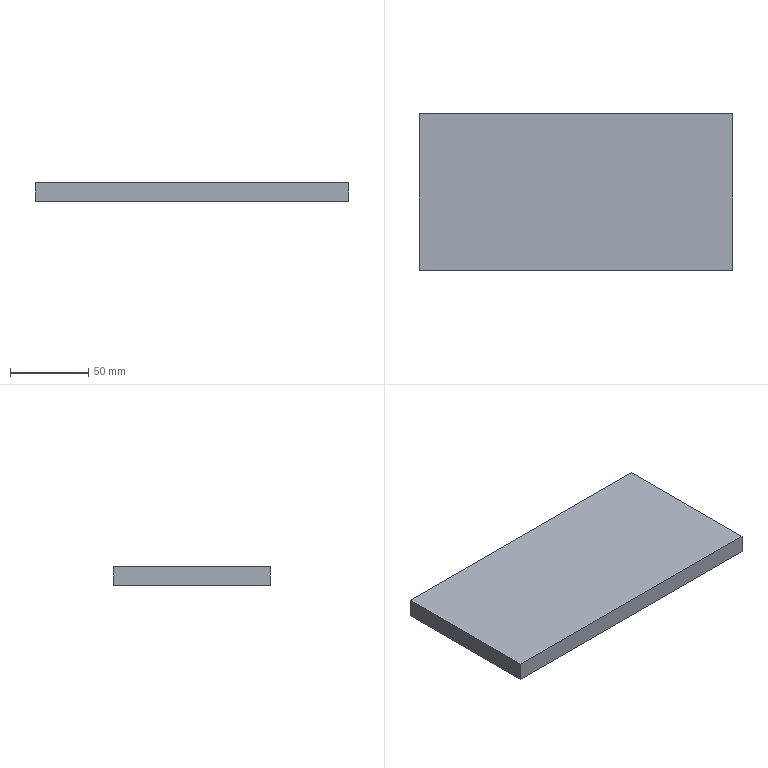Part | SolidWorks | features Extrusion 1 | 1 solid | 6 faces | box 200 x 100 x 12 mm | volume 240000 mm3 | plane 6
STEP:
#1=CARTESIAN_POINT('',(100.,-50.,0.));
#2=VERTEX_POINT('',#1);
#3=CARTESIAN_POINT('',(100.,50.,0.));
#4=VERTEX_POINT('',#3);
#5=CARTESIAN_POINT('',(100.,-50.,0.));
#6=DIRECTION('',(0.,1.,0.));
#7=VECTOR('',#6,1000.);
#8=LINE('',#5,#7);
#9=EDGE_CURVE('',#2,#4,#8,.T.);
#10=ORIENTED_EDGE('',*,*,#9,.T.);
#11=CARTESIAN_POINT('',(100.,50.,12.));
#12=VERTEX_POINT('',#11);
#13=CARTESIAN_POINT('',(100.,50.,12.));
#14=DIRECTION('',(0.,0.,-1.));
#15=VECTOR('',#14,1000.);
#16=LINE('',#13,#15);
#17=EDGE_CURVE('',#12,#4,#16,.T.);
#18=ORIENTED_EDGE('',*,*,#17,.F.);
#19=CARTESIAN_POINT('',(100.,-50.,12.));
#20=VERTEX_POINT('',#19);
#21=CARTESIAN_POINT('',(100.,-50.,12.));
#22=DIRECTION('',(0.,1.,0.));
#23=VECTOR('',#22,1000.);
#24=LINE('',#21,#23);
#25=EDGE_CURVE('',#20,#12,#24,.T.);
#26=ORIENTED_EDGE('',*,*,#25,.F.);
#27=CARTESIAN_POINT('',(100.,-50.,12.));
#28=DIRECTION('',(0.,0.,-1.));
#29=VECTOR('',#28,1000.);
#30=LINE('',#27,#29);
#31=EDGE_CURVE('',#20,#2,#30,.T.);
#32=ORIENTED_EDGE('',*,*,#31,.T.);
#33=EDGE_LOOP('',(#10,#18,#26,#32));
#34=FACE_OUTER_BOUND('',#33,.T.);
#35=CARTESIAN_POINT('',(100.,-50.,12.));
#36=DIRECTION('',(-1.,0.,0.));
#37=DIRECTION('',(0.,0.,1.));
#38=AXIS2_PLACEMENT_3D('',#35,#36,#37);
#39=PLANE('',#38);
#40=ADVANCED_FACE('',(#34),#39,.F.);
#41=CARTESIAN_POINT('',(-100.,50.,0.));
#42=VERTEX_POINT('',#41);
#43=CARTESIAN_POINT('',(-100.,50.,0.));
#44=DIRECTION('',(-1.,0.,0.));
#45=VECTOR('',#44,1000.);
#46=LINE('',#43,#45);
#47=EDGE_CURVE('',#4,#42,#46,.T.);
#48=ORIENTED_EDGE('',*,*,#47,.T.);
#49=CARTESIAN_POINT('',(-100.,50.,12.));
#50=VERTEX_POINT('',#49);
#51=CARTESIAN_POINT('',(-100.,50.,12.));
#52=DIRECTION('',(0.,0.,-1.));
#53=VECTOR('',#52,1000.);
#54=LINE('',#51,#53);
#55=EDGE_CURVE('',#50,#42,#54,.T.);
#56=ORIENTED_EDGE('',*,*,#55,.F.);
#57=CARTESIAN_POINT('',(-100.,50.,12.));
#58=DIRECTION('',(-1.,0.,0.));
#59=VECTOR('',#58,1000.);
#60=LINE('',#57,#59);
#61=EDGE_CURVE('',#12,#50,#60,.T.);
#62=ORIENTED_EDGE('',*,*,#61,.F.);
#63=ORIENTED_EDGE('',*,*,#17,.T.);
#64=EDGE_LOOP('',(#48,#56,#62,#63));
#65=FACE_OUTER_BOUND('',#64,.T.);
#66=CARTESIAN_POINT('',(-100.,50.,12.));
#67=DIRECTION('',(0.,-1.,0.));
#68=DIRECTION('',(0.,0.,-1.));
#69=AXIS2_PLACEMENT_3D('',#66,#67,#68);
#70=PLANE('',#69);
#71=ADVANCED_FACE('',(#65),#70,.F.);
#72=CARTESIAN_POINT('',(-100.,-50.,0.));
#73=VERTEX_POINT('',#72);
#74=CARTESIAN_POINT('',(-100.,-50.,0.));
#75=DIRECTION('',(0.,-1.,0.));
#76=VECTOR('',#75,1000.);
#77=LINE('',#74,#76);
#78=EDGE_CURVE('',#42,#73,#77,.T.);
#79=ORIENTED_EDGE('',*,*,#78,.T.);
#80=CARTESIAN_POINT('',(-100.,-50.,12.));
#81=VERTEX_POINT('',#80);
#82=CARTESIAN_POINT('',(-100.,-50.,12.));
#83=DIRECTION('',(0.,0.,-1.));
#84=VECTOR('',#83,1000.);
#85=LINE('',#82,#84);
#86=EDGE_CURVE('',#81,#73,#85,.T.);
#87=ORIENTED_EDGE('',*,*,#86,.F.);
#88=CARTESIAN_POINT('',(-100.,-50.,12.));
#89=DIRECTION('',(0.,-1.,0.));
#90=VECTOR('',#89,1000.);
#91=LINE('',#88,#90);
#92=EDGE_CURVE('',#50,#81,#91,.T.);
#93=ORIENTED_EDGE('',*,*,#92,.F.);
#94=ORIENTED_EDGE('',*,*,#55,.T.);
#95=EDGE_LOOP('',(#79,#87,#93,#94));
#96=FACE_OUTER_BOUND('',#95,.T.);
#97=CARTESIAN_POINT('',(-100.,-50.,12.));
#98=DIRECTION('',(1.,0.,0.));
#99=DIRECTION('',(0.,0.,-1.));
#100=AXIS2_PLACEMENT_3D('',#97,#98,#99);
#101=PLANE('',#100);
#102=ADVANCED_FACE('',(#96),#101,.F.);
#103=CARTESIAN_POINT('',(-100.,-50.,0.));
#104=DIRECTION('',(1.,0.,0.));
#105=VECTOR('',#104,1000.);
#106=LINE('',#103,#105);
#107=EDGE_CURVE('',#73,#2,#106,.T.);
#108=ORIENTED_EDGE('',*,*,#107,.T.);
#109=ORIENTED_EDGE('',*,*,#31,.F.);
#110=CARTESIAN_POINT('',(-100.,-50.,12.));
#111=DIRECTION('',(1.,0.,0.));
#112=VECTOR('',#111,1000.);
#113=LINE('',#110,#112);
#114=EDGE_CURVE('',#81,#20,#113,.T.);
#115=ORIENTED_EDGE('',*,*,#114,.F.);
#116=ORIENTED_EDGE('',*,*,#86,.T.);
#117=EDGE_LOOP('',(#108,#109,#115,#116));
#118=FACE_OUTER_BOUND('',#117,.T.);
#119=CARTESIAN_POINT('',(-100.,-50.,12.));
#120=DIRECTION('',(0.,1.,0.));
#121=DIRECTION('',(0.,0.,1.));
#122=AXIS2_PLACEMENT_3D('',#119,#120,#121);
#123=PLANE('',#122);
#124=ADVANCED_FACE('',(#118),#123,.F.);
#125=ORIENTED_EDGE('',*,*,#25,.T.);
#126=ORIENTED_EDGE('',*,*,#61,.T.);
#127=ORIENTED_EDGE('',*,*,#92,.T.);
#128=ORIENTED_EDGE('',*,*,#114,.T.);
#129=EDGE_LOOP('',(#125,#126,#127,#128));
#130=FACE_OUTER_BOUND('',#129,.T.);
#131=CARTESIAN_POINT('',(0.,0.,12.));
#132=DIRECTION('',(0.,0.,-1.));
#133=DIRECTION('',(-1.,0.,0.));
#134=AXIS2_PLACEMENT_3D('',#131,#132,#133);
#135=PLANE('',#134);
#136=ADVANCED_FACE('',(#130),#135,.F.);
#137=ORIENTED_EDGE('',*,*,#9,.F.);
#138=ORIENTED_EDGE('',*,*,#107,.F.);
#139=ORIENTED_EDGE('',*,*,#78,.F.);
#140=ORIENTED_EDGE('',*,*,#47,.F.);
#141=EDGE_LOOP('',(#137,#138,#139,#140));
#142=FACE_OUTER_BOUND('',#141,.T.);
#143=CARTESIAN_POINT('',(0.,0.,0.));
#144=DIRECTION('',(0.,0.,-1.));
#145=DIRECTION('',(-1.,0.,0.));
#146=AXIS2_PLACEMENT_3D('',#143,#144,#145);
#147=PLANE('',#146);
#148=ADVANCED_FACE('',(#142),#147,.T.);
#149=CLOSED_SHELL('',(#40,#71,#102,#124,#136,#148));
#150=MANIFOLD_SOLID_BREP('',#149);
#151=CARTESIAN_POINT('',(0.,0.,0.));
#152=DIRECTION('',(0.,0.,1.));
#153=DIRECTION('',(1.,0.,0.));
#154=AXIS2_PLACEMENT_3D('',#151,#152,#153);
#155=(LENGTH_UNIT()NAMED_UNIT(*)SI_UNIT(.MILLI.,.METRE.));
#156=UNCERTAINTY_MEASURE_WITH_UNIT(LENGTH_MEASURE(0.00001),#155,'','');
#157=(NAMED_UNIT(*)PLANE_ANGLE_UNIT()SI_UNIT($,.RADIAN.));
#158=(NAMED_UNIT(*)SI_UNIT($,.STERADIAN.)SOLID_ANGLE_UNIT());
#159=(GEOMETRIC_REPRESENTATION_CONTEXT(3)GLOBAL_UNCERTAINTY_ASSIGNED_CONTEXT((#156))GLOBAL_UNIT_ASSIGNED_CONTEXT((#155,#157,#158))REPRESENTATION_CONTEXT('',''));
#160=ADVANCED_BREP_SHAPE_REPRESENTATION('',(#150,#154),#159);